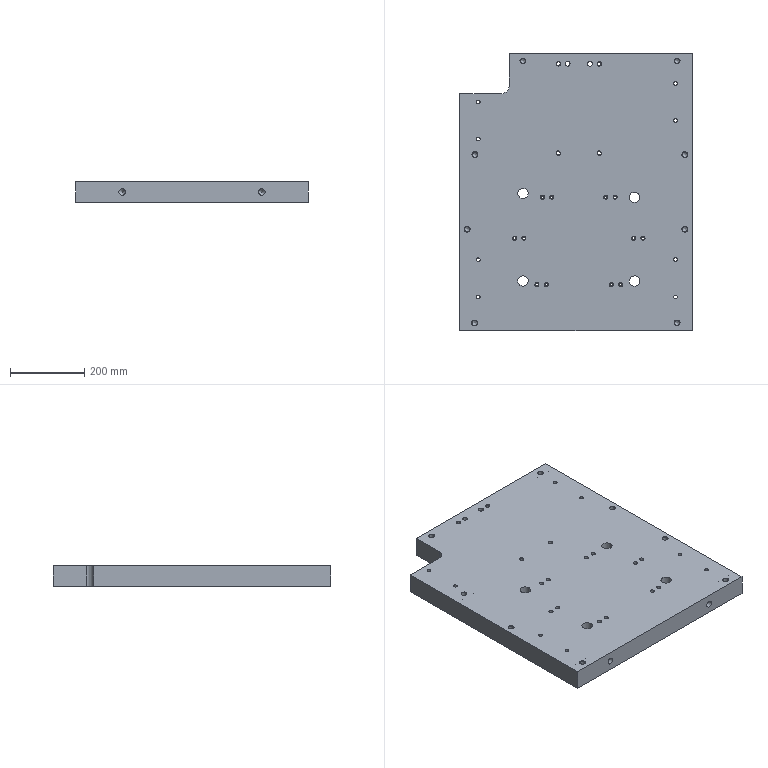Part | NX | features solid 2 | 1 solid | 231 faces | box 625 x 745 x 55 mm | volume 22288617 mm3 | cylinder 97 | cone 92 | plane 34 | spline 8 | commonest cylinder face diameters 8.5 x22 14 x16 7 x12 11 x12 40 x9 10 x8